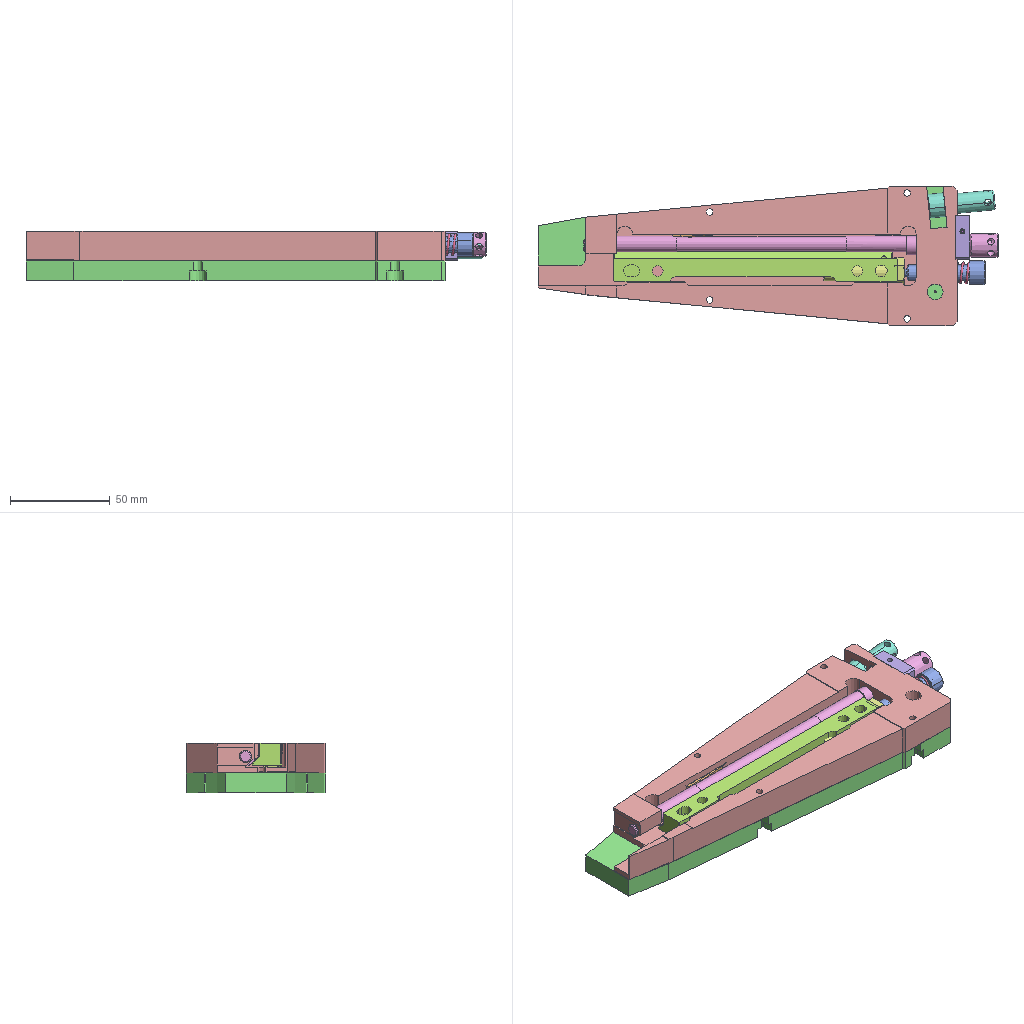Assembly | SolidWorks | 14 different items | 18 placed | box 231 x 70 x 25 mm
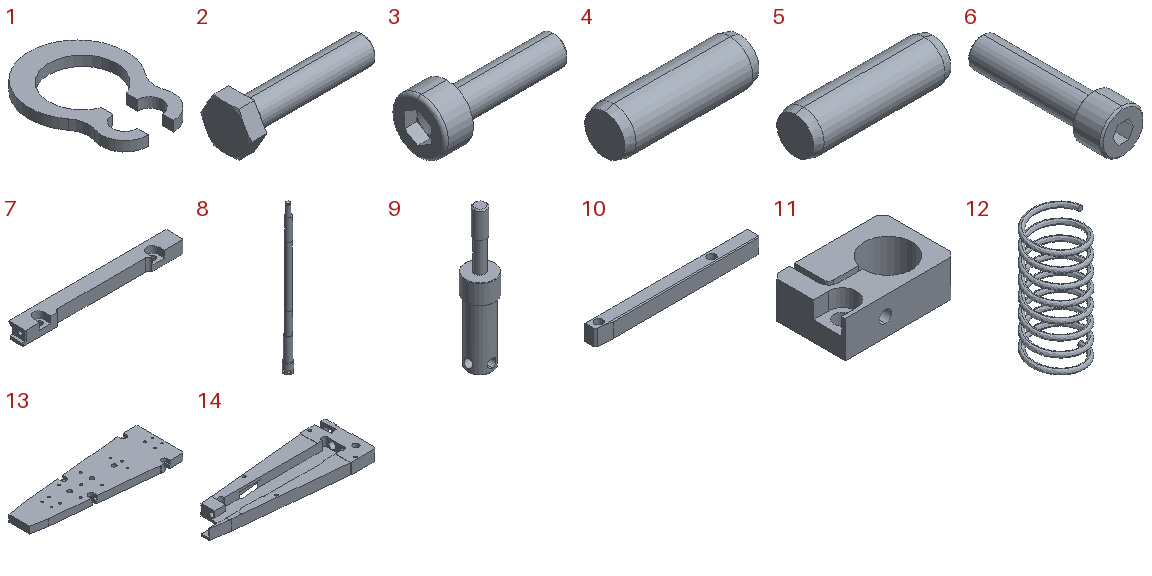Parts list (item | quantity | size | volume | features):
1 | x1 | 3.9 x 5.304 x 0.4 mm | 3.093 mm3 | features Boss 1
2 | x1 | 40.3 x 15.011 x 13 mm | 2514 mm3 | features RevCut 3, Boss 1, Chamfer 1, Extrusion 1, Fillet 1, LPattern 1
3 | x2 | 7.6 x 3 x 3 mm | 21.652 mm3 | features Fillet 2, RevCut 2, Boss 1, Chamfer 1, Cut 1, Extrusion 1, LPattern 1
4 | x3 | 3 x 1 x 1 mm | 2.324 mm3 | features Revolution 1
5 | x2 | 2 x 0.6 x 0.6 mm | 0.5585 mm3 | features Revolution 1
6 | x1 | 12 x 40.5 x 12 mm | 2375 mm3 | features ICE 4, Chamfer 2, CirPattern 1, Extrusion 1, Fillet 1, RevCut 1
7 | x1 | 142 x 15 x 11 mm | 15061 mm3 | features ICE 7, Chamfer 3, HoleWzd 2, Extrusion 1
8 | x1 | 12 x 12 x 207.5 mm | 10807 mm3 | features ICE 6, Chamfer 2, CirPattern 1, Extrusion 1, RevCut 1
9 | x1 | 11.9 x 11.9 x 56 mm | 3013 mm3 | features ICE 5, Chamfer 2, CirPattern 1, Extrusion 1, Fillet 1
10 | x1 | 101 x 8 x 10 mm | 7248 mm3 | features Chamfer 2, Extrusion 1, HoleWzd 1, ICE 1
11 | x1 | 22 x 14.5 x 7.3 mm | 1409 mm3 | features ICE 4, HoleWzd 3, Fillet 2, Chamfer 1, Extrusion 1
12 | x1 | 11 x 11 x 25 mm | 196.371 mm3 | features Helix 1, RefAxis 1, Sweep 1
13 | x1 | 210 x 70 x 10 mm | 108255 mm3 | features HoleWzd 5, ICE 5, Chamfer 2, Cut 1, Extrusion 1
14 | x1 | 210 x 70 x 15 mm | 86149 mm3 | features ICE 13, Chamfer 2, Fillet 2, HoleWzd 2, Extrusion 1
Mates (type | each side: item.copy, entity, surface, feature):
Concentric | 14.1 face cylinder Cut-Extrude6 | 6.1 face cylinder Boss-Extrude2
DistanceDim | 14.1 face plane Boss-Extrude1 | 6.1 face plane Boss-Extrude1
Parallel | 14.1 face plane Cut-Extrude10 | 7.1 face plane Boss-Extrude1
Concentric | 6.1 face cylinder Boss-Extrude2 | 7.1 face cylinder M4 Tapped Hole1
Concentric | 14.1 face cylinder Cut-Extrude6 | 8.1 face cylinder Boss-Extrude2
Coincident | 14.1 face plane Cut-Extrude1 | 9.1 face plane Boss-Extrude2
Parallel | 14.1 face plane Cut-Extrude5 | 10.1 face plane Boss-Extrude1
Coincident | 14.1 face plane Boss-Extrude1 | 13.1 face plane Boss-Extrude2 | 3 times
Coincident | 6.1 plane | 12.1 plane
Concentric | 6.1 face cylinder Boss-Extrude2 | 12.1 axis
Coincident | 14.1 face plane Cut-Extrude14 | 10.1 face plane Boss-Extrude1
Concentric | 8.1 face cylinder Cut-Revolve1 | 1.1 face cylinder Body
Coincident | 8.1 face plane Cut-Revolve1 | 1.1 face plane Body
Coincident | 11.1 face plane Boss-Extrude1 | 14.1 face plane Cut-Extrude18
Concentric | 8.1 face cylinder Boss-Extrude2 | 11.1 face cylinder Cut-Extrude1
Parallel | 14.1 face plane Cut-Extrude5 | 11.1 face plane Boss-Extrude1
Concentric | 2.1 face cylinder BaseBody | 7.1 face cylinder M4 Tapped Hole1
Coincident | 6.1 face plane Boss-Extrude3 | 2.1 face plane BaseHead
Concentric | 11.1 face cylinder Hole size per socket head cap screw type 3 | 3.1 face cylinder BaseBody
Coincident | 11.1 face plane Hole size per socket head cap screw type 3 | 3.1 face plane BaseHead
Concentric | 11.1 face cylinder Ø3.4 (3.4) Diameter Hole1 | 3.2 face cylinder BaseBody
Coincident | 11.1 face plane Cut-Extrude4 | 3.2 face plane BaseHead
Concentric | 14.1 face cylinder Cut-Extrude1 | 4.1 face cylinder Base-Revolve
DistanceDim | 4.1 face plane Base-Revolve | 14.1 face plane Cut-Extrude5
Concentric | 9.1 face cylinder Boss-Extrude4 | 10.1 face cylinder M5 Tapped Hole1
Coincident | 14.1 face plane Cut-Extrude14 | 4.2 face plane Base-Revolve
Concentric | 10.1 face cylinder Cut-Extrude1 | 4.2 face cylinder Base-Revolve
Coincident | 14.1 face plane Cut-Extrude14 | 4.3 face plane Base-Revolve
Concentric | 10.1 face cylinder Cut-Extrude1 | 4.3 face cylinder Base-Revolve
Tangent | 13.1 face plane Cut-Extrude4 | 4.2 face cylinder Base-Revolve
Coincident | 14.1 face plane Cut-Extrude5 | 10.1 face plane Boss-Extrude1
DistanceDim | 7.1 face plane Cut-Extrude4 | 14.1 face plane Cut-Extrude2
Coincident | 14.1 face plane Cut-Extrude17 | 8.1 face plane Cut-Revolve1
Concentric | 13.1 face cylinder Cut-Extrude6 | 5.1 face cylinder Base-Revolve
Concentric | 13.1 face cylinder Cut-Extrude6 | 5.2 face cylinder Base-Revolve
Coincident | 13.1 face plane Cut-Extrude6 | 5.1 face plane Base-Revolve
Coincident | 5.1 face plane Base-Revolve | 5.2 face plane Base-Revolve